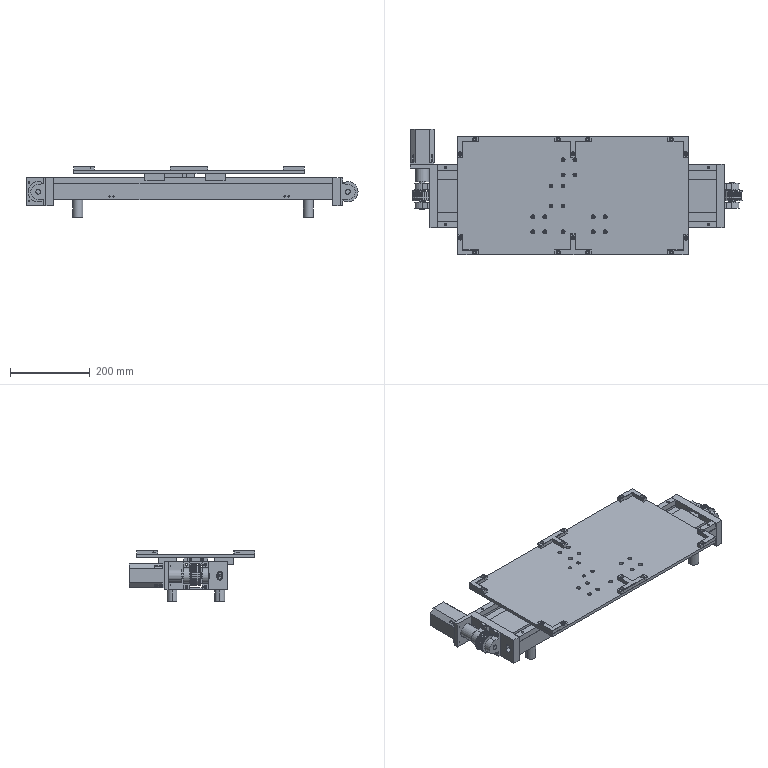Part | 36 solids | 1265 faces | box 834.5 x 316.5 x 128 mm | volume 6961045 mm3 | cylinder 709 | plane 448 | cone 108 | commonest cylinder face diameters 0.96 x140 1.14 x80 3.3 x64 47.75 x62 5 x56 6 x56